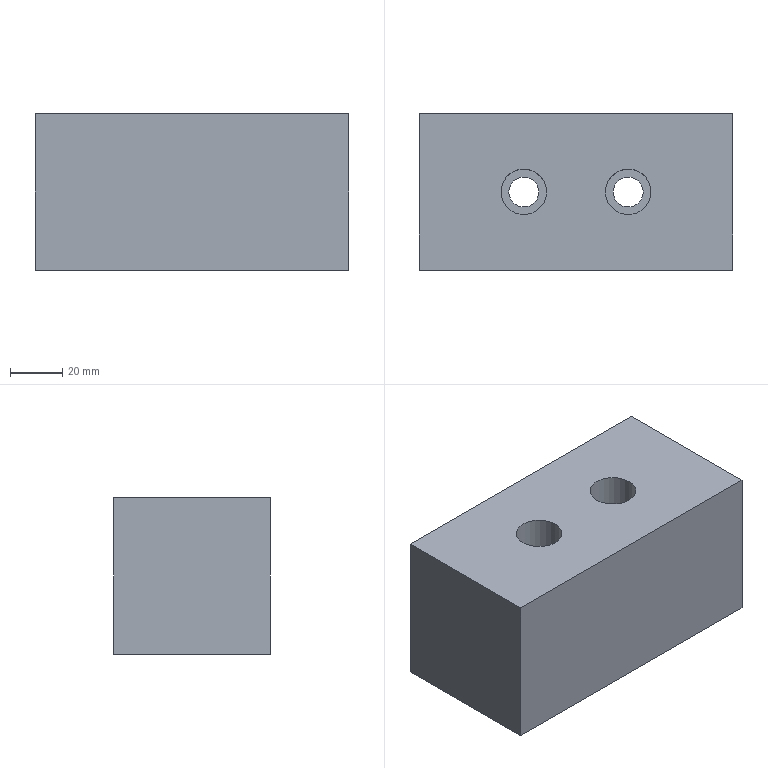Part | NX | features solid 2 | 1 solid | 12 faces | box 120 x 60 x 60 mm | volume 408603 mm3 | plane 8 | cylinder 4 | commonest cylinder face diameters 11.5 x2 17.5 x2
STEP:
#1=CARTESIAN_POINT('',(1280.,-260.,55.));
#2=VERTEX_POINT('',#1);
#3=CARTESIAN_POINT('',(1160.,-260.,55.));
#4=VERTEX_POINT('',#3);
#5=CARTESIAN_POINT('',(1295.,-260.,55.));
#6=DIRECTION('',(-1.,0.,0.));
#7=VECTOR('',#6,1000.);
#8=LINE('',#5,#7);
#9=EDGE_CURVE('',#2,#4,#8,.T.);
#10=ORIENTED_EDGE('',*,*,#9,.F.);
#11=CARTESIAN_POINT('',(1280.,-260.,-5.));
#12=VERTEX_POINT('',#11);
#13=CARTESIAN_POINT('',(1280.,-260.,-5.));
#14=DIRECTION('',(0.,0.,1.));
#15=VECTOR('',#14,1000.);
#16=LINE('',#13,#15);
#17=EDGE_CURVE('',#12,#2,#16,.T.);
#18=ORIENTED_EDGE('',*,*,#17,.F.);
#19=CARTESIAN_POINT('',(1160.,-260.,-5.));
#20=VERTEX_POINT('',#19);
#21=CARTESIAN_POINT('',(1295.,-260.,-5.));
#22=DIRECTION('',(-1.,0.,0.));
#23=VECTOR('',#22,1000.);
#24=LINE('',#21,#23);
#25=EDGE_CURVE('',#12,#20,#24,.T.);
#26=ORIENTED_EDGE('',*,*,#25,.T.);
#27=CARTESIAN_POINT('',(1160.,-260.,-5.));
#28=DIRECTION('',(0.,0.,1.));
#29=VECTOR('',#28,1000.);
#30=LINE('',#27,#29);
#31=EDGE_CURVE('',#20,#4,#30,.T.);
#32=ORIENTED_EDGE('',*,*,#31,.T.);
#33=EDGE_LOOP('',(#10,#18,#26,#32));
#34=FACE_BOUND('',#33,.T.);
#35=CARTESIAN_POINT('',(1295.,-260.,-5.));
#36=DIRECTION('',(0.,1.,0.));
#37=DIRECTION('',(0.,0.,1.));
#38=AXIS2_PLACEMENT_3D('',#35,#36,#37);
#39=PLANE('',#38);
#40=ADVANCED_FACE('',(#34),#39,.T.);
#41=CARTESIAN_POINT('',(1160.,-320.,55.));
#42=VERTEX_POINT('',#41);
#43=CARTESIAN_POINT('',(1160.,-335.,55.));
#44=DIRECTION('',(0.,1.,0.));
#45=VECTOR('',#44,1000.);
#46=LINE('',#43,#45);
#47=EDGE_CURVE('',#42,#4,#46,.T.);
#48=ORIENTED_EDGE('',*,*,#47,.T.);
#49=ORIENTED_EDGE('',*,*,#31,.F.);
#50=CARTESIAN_POINT('',(1160.,-320.,-5.));
#51=VERTEX_POINT('',#50);
#52=CARTESIAN_POINT('',(1160.,-335.,-5.));
#53=DIRECTION('',(0.,1.,0.));
#54=VECTOR('',#53,1000.);
#55=LINE('',#52,#54);
#56=EDGE_CURVE('',#51,#20,#55,.T.);
#57=ORIENTED_EDGE('',*,*,#56,.F.);
#58=CARTESIAN_POINT('',(1160.,-320.,-5.));
#59=DIRECTION('',(0.,0.,1.));
#60=VECTOR('',#59,1000.);
#61=LINE('',#58,#60);
#62=EDGE_CURVE('',#51,#42,#61,.T.);
#63=ORIENTED_EDGE('',*,*,#62,.T.);
#64=EDGE_LOOP('',(#48,#49,#57,#63));
#65=FACE_BOUND('',#64,.T.);
#66=CARTESIAN_POINT('',(1160.,-335.,-5.));
#67=DIRECTION('',(1.,0.,0.));
#68=DIRECTION('',(0.,0.,-1.));
#69=AXIS2_PLACEMENT_3D('',#66,#67,#68);
#70=PLANE('',#69);
#71=ADVANCED_FACE('',(#65),#70,.F.);
#72=CARTESIAN_POINT('',(1280.,-320.,55.));
#73=VERTEX_POINT('',#72);
#74=CARTESIAN_POINT('',(1295.,-320.,55.));
#75=DIRECTION('',(-1.,0.,0.));
#76=VECTOR('',#75,1000.);
#77=LINE('',#74,#76);
#78=EDGE_CURVE('',#73,#42,#77,.T.);
#79=ORIENTED_EDGE('',*,*,#78,.T.);
#80=ORIENTED_EDGE('',*,*,#62,.F.);
#81=CARTESIAN_POINT('',(1280.,-320.,-5.));
#82=VERTEX_POINT('',#81);
#83=CARTESIAN_POINT('',(1295.,-320.,-5.));
#84=DIRECTION('',(-1.,0.,0.));
#85=VECTOR('',#84,1000.);
#86=LINE('',#83,#85);
#87=EDGE_CURVE('',#82,#51,#86,.T.);
#88=ORIENTED_EDGE('',*,*,#87,.F.);
#89=CARTESIAN_POINT('',(1280.,-320.,-5.));
#90=DIRECTION('',(0.,0.,1.));
#91=VECTOR('',#90,1000.);
#92=LINE('',#89,#91);
#93=EDGE_CURVE('',#82,#73,#92,.T.);
#94=ORIENTED_EDGE('',*,*,#93,.T.);
#95=EDGE_LOOP('',(#79,#80,#88,#94));
#96=FACE_BOUND('',#95,.T.);
#97=CARTESIAN_POINT('',(1295.,-320.,-5.));
#98=DIRECTION('',(0.,1.,0.));
#99=DIRECTION('',(0.,0.,1.));
#100=AXIS2_PLACEMENT_3D('',#97,#98,#99);
#101=PLANE('',#100);
#102=ADVANCED_FACE('',(#96),#101,.F.);
#103=CARTESIAN_POINT('',(1280.,-335.,55.));
#104=DIRECTION('',(0.,1.,0.));
#105=VECTOR('',#104,1000.);
#106=LINE('',#103,#105);
#107=EDGE_CURVE('',#73,#2,#106,.T.);
#108=ORIENTED_EDGE('',*,*,#107,.F.);
#109=ORIENTED_EDGE('',*,*,#93,.F.);
#110=CARTESIAN_POINT('',(1280.,-335.,-5.));
#111=DIRECTION('',(0.,1.,0.));
#112=VECTOR('',#111,1000.);
#113=LINE('',#110,#112);
#114=EDGE_CURVE('',#82,#12,#113,.T.);
#115=ORIENTED_EDGE('',*,*,#114,.T.);
#116=ORIENTED_EDGE('',*,*,#17,.T.);
#117=EDGE_LOOP('',(#108,#109,#115,#116));
#118=FACE_BOUND('',#117,.T.);
#119=CARTESIAN_POINT('',(1280.,-335.,-5.));
#120=DIRECTION('',(1.,0.,0.));
#121=DIRECTION('',(0.,0.,-1.));
#122=AXIS2_PLACEMENT_3D('',#119,#120,#121);
#123=PLANE('',#122);
#124=ADVANCED_FACE('',(#118),#123,.T.);
#125=CARTESIAN_POINT('',(1194.25,-290.,-5.));
#126=VERTEX_POINT('',#125);
#127=CARTESIAN_POINT('',(1200.,-290.,-5.));
#128=DIRECTION('',(0.,0.,-1.));
#129=DIRECTION('',(-1.,0.,0.));
#130=AXIS2_PLACEMENT_3D('',#127,#128,#129);
#131=CIRCLE('',#130,5.75);
#132=EDGE_CURVE('',#126,#126,#131,.T.);
#133=ORIENTED_EDGE('',*,*,#132,.F.);
#134=EDGE_LOOP('',(#133));
#135=FACE_BOUND('',#134,.T.);
#136=CARTESIAN_POINT('',(1234.25,-290.,-5.));
#137=VERTEX_POINT('',#136);
#138=CARTESIAN_POINT('',(1240.,-290.,-5.));
#139=DIRECTION('',(0.,0.,-1.));
#140=DIRECTION('',(-1.,0.,0.));
#141=AXIS2_PLACEMENT_3D('',#138,#139,#140);
#142=CIRCLE('',#141,5.75);
#143=EDGE_CURVE('',#137,#137,#142,.T.);
#144=ORIENTED_EDGE('',*,*,#143,.F.);
#145=EDGE_LOOP('',(#144));
#146=FACE_BOUND('',#145,.T.);
#147=ORIENTED_EDGE('',*,*,#25,.F.);
#148=ORIENTED_EDGE('',*,*,#114,.F.);
#149=ORIENTED_EDGE('',*,*,#87,.T.);
#150=ORIENTED_EDGE('',*,*,#56,.T.);
#151=EDGE_LOOP('',(#147,#148,#149,#150));
#152=FACE_BOUND('',#151,.T.);
#153=CARTESIAN_POINT('',(1295.,-335.,-5.));
#154=DIRECTION('',(0.,0.,-1.));
#155=DIRECTION('',(-1.,0.,0.));
#156=AXIS2_PLACEMENT_3D('',#153,#154,#155);
#157=PLANE('',#156);
#158=ADVANCED_FACE('',(#135,#146,#152),#157,.T.);
#159=CARTESIAN_POINT('',(1191.25,-290.,55.));
#160=VERTEX_POINT('',#159);
#161=CARTESIAN_POINT('',(1200.,-290.,55.));
#162=DIRECTION('',(0.,0.,1.));
#163=DIRECTION('',(-1.,0.,0.));
#164=AXIS2_PLACEMENT_3D('',#161,#162,#163);
#165=CIRCLE('',#164,8.75);
#166=EDGE_CURVE('',#160,#160,#165,.F.);
#167=ORIENTED_EDGE('',*,*,#166,.T.);
#168=EDGE_LOOP('',(#167));
#169=FACE_BOUND('',#168,.T.);
#170=CARTESIAN_POINT('',(1231.25,-290.,55.));
#171=VERTEX_POINT('',#170);
#172=CARTESIAN_POINT('',(1240.,-290.,55.));
#173=DIRECTION('',(0.,0.,1.));
#174=DIRECTION('',(-1.,0.,0.));
#175=AXIS2_PLACEMENT_3D('',#172,#173,#174);
#176=CIRCLE('',#175,8.75);
#177=EDGE_CURVE('',#171,#171,#176,.F.);
#178=ORIENTED_EDGE('',*,*,#177,.T.);
#179=EDGE_LOOP('',(#178));
#180=FACE_BOUND('',#179,.T.);
#181=ORIENTED_EDGE('',*,*,#9,.T.);
#182=ORIENTED_EDGE('',*,*,#47,.F.);
#183=ORIENTED_EDGE('',*,*,#78,.F.);
#184=ORIENTED_EDGE('',*,*,#107,.T.);
#185=EDGE_LOOP('',(#181,#182,#183,#184));
#186=FACE_BOUND('',#185,.T.);
#187=CARTESIAN_POINT('',(1295.,-335.,55.));
#188=DIRECTION('',(0.,0.,-1.));
#189=DIRECTION('',(-1.,0.,0.));
#190=AXIS2_PLACEMENT_3D('',#187,#188,#189);
#191=PLANE('',#190);
#192=ADVANCED_FACE('',(#169,#180,#186),#191,.F.);
#193=ORIENTED_EDGE('',*,*,#143,.T.);
#194=EDGE_LOOP('',(#193));
#195=FACE_BOUND('',#194,.T.);
#196=CARTESIAN_POINT('',(1234.25,-290.,15.));
#197=VERTEX_POINT('',#196);
#198=CARTESIAN_POINT('',(1240.,-290.,15.));
#199=DIRECTION('',(0.,0.,-1.));
#200=DIRECTION('',(-1.,0.,0.));
#201=AXIS2_PLACEMENT_3D('',#198,#199,#200);
#202=CIRCLE('',#201,5.75);
#203=EDGE_CURVE('',#197,#197,#202,.T.);
#204=ORIENTED_EDGE('',*,*,#203,.F.);
#205=EDGE_LOOP('',(#204));
#206=FACE_BOUND('',#205,.T.);
#207=CARTESIAN_POINT('',(1240.,-290.,-25.));
#208=DIRECTION('',(0.,0.,-1.));
#209=DIRECTION('',(-1.,0.,0.));
#210=AXIS2_PLACEMENT_3D('',#207,#208,#209);
#211=CYLINDRICAL_SURFACE('',#210,5.75);
#212=ADVANCED_FACE('',(#195,#206),#211,.F.);
#213=ORIENTED_EDGE('',*,*,#203,.T.);
#214=EDGE_LOOP('',(#213));
#215=FACE_BOUND('',#214,.T.);
#216=CARTESIAN_POINT('',(1231.25,-290.,15.));
#217=VERTEX_POINT('',#216);
#218=CARTESIAN_POINT('',(1240.,-290.,15.));
#219=DIRECTION('',(0.,0.,-1.));
#220=DIRECTION('',(-1.,0.,0.));
#221=AXIS2_PLACEMENT_3D('',#218,#219,#220);
#222=CIRCLE('',#221,8.75);
#223=EDGE_CURVE('',#217,#217,#222,.T.);
#224=ORIENTED_EDGE('',*,*,#223,.F.);
#225=EDGE_LOOP('',(#224));
#226=FACE_BOUND('',#225,.T.);
#227=CARTESIAN_POINT('',(1240.,-290.,15.));
#228=DIRECTION('',(0.,0.,-1.));
#229=DIRECTION('',(-1.,0.,0.));
#230=AXIS2_PLACEMENT_3D('',#227,#228,#229);
#231=PLANE('',#230);
#232=ADVANCED_FACE('',(#215,#226),#231,.F.);
#233=ORIENTED_EDGE('',*,*,#223,.T.);
#234=EDGE_LOOP('',(#233));
#235=FACE_BOUND('',#234,.T.);
#236=ORIENTED_EDGE('',*,*,#177,.F.);
#237=EDGE_LOOP('',(#236));
#238=FACE_BOUND('',#237,.T.);
#239=CARTESIAN_POINT('',(1240.,-290.,65.));
#240=DIRECTION('',(0.,0.,-1.));
#241=DIRECTION('',(-1.,0.,0.));
#242=AXIS2_PLACEMENT_3D('',#239,#240,#241);
#243=CYLINDRICAL_SURFACE('',#242,8.75);
#244=ADVANCED_FACE('',(#235,#238),#243,.F.);
#245=ORIENTED_EDGE('',*,*,#132,.T.);
#246=EDGE_LOOP('',(#245));
#247=FACE_BOUND('',#246,.T.);
#248=CARTESIAN_POINT('',(1194.25,-290.,15.));
#249=VERTEX_POINT('',#248);
#250=CARTESIAN_POINT('',(1200.,-290.,15.));
#251=DIRECTION('',(0.,0.,-1.));
#252=DIRECTION('',(-1.,0.,0.));
#253=AXIS2_PLACEMENT_3D('',#250,#251,#252);
#254=CIRCLE('',#253,5.75);
#255=EDGE_CURVE('',#249,#249,#254,.T.);
#256=ORIENTED_EDGE('',*,*,#255,.F.);
#257=EDGE_LOOP('',(#256));
#258=FACE_BOUND('',#257,.T.);
#259=CARTESIAN_POINT('',(1200.,-290.,-25.));
#260=DIRECTION('',(0.,0.,-1.));
#261=DIRECTION('',(-1.,0.,0.));
#262=AXIS2_PLACEMENT_3D('',#259,#260,#261);
#263=CYLINDRICAL_SURFACE('',#262,5.75);
#264=ADVANCED_FACE('',(#247,#258),#263,.F.);
#265=ORIENTED_EDGE('',*,*,#255,.T.);
#266=EDGE_LOOP('',(#265));
#267=FACE_BOUND('',#266,.T.);
#268=CARTESIAN_POINT('',(1191.25,-290.,15.));
#269=VERTEX_POINT('',#268);
#270=CARTESIAN_POINT('',(1200.,-290.,15.));
#271=DIRECTION('',(0.,0.,-1.));
#272=DIRECTION('',(-1.,0.,0.));
#273=AXIS2_PLACEMENT_3D('',#270,#271,#272);
#274=CIRCLE('',#273,8.75);
#275=EDGE_CURVE('',#269,#269,#274,.T.);
#276=ORIENTED_EDGE('',*,*,#275,.F.);
#277=EDGE_LOOP('',(#276));
#278=FACE_BOUND('',#277,.T.);
#279=CARTESIAN_POINT('',(1200.,-290.,15.));
#280=DIRECTION('',(0.,0.,-1.));
#281=DIRECTION('',(-1.,0.,0.));
#282=AXIS2_PLACEMENT_3D('',#279,#280,#281);
#283=PLANE('',#282);
#284=ADVANCED_FACE('',(#267,#278),#283,.F.);
#285=ORIENTED_EDGE('',*,*,#275,.T.);
#286=EDGE_LOOP('',(#285));
#287=FACE_BOUND('',#286,.T.);
#288=ORIENTED_EDGE('',*,*,#166,.F.);
#289=EDGE_LOOP('',(#288));
#290=FACE_BOUND('',#289,.T.);
#291=CARTESIAN_POINT('',(1200.,-290.,65.));
#292=DIRECTION('',(0.,0.,-1.));
#293=DIRECTION('',(-1.,0.,0.));
#294=AXIS2_PLACEMENT_3D('',#291,#292,#293);
#295=CYLINDRICAL_SURFACE('',#294,8.75);
#296=ADVANCED_FACE('',(#287,#290),#295,.F.);
#297=CLOSED_SHELL('',(#40,#71,#102,#124,#158,#192,#212,#232,#244,#264,#284,#296));
#298=MANIFOLD_SOLID_BREP('',#297);
#299=(LENGTH_UNIT()NAMED_UNIT(*)SI_UNIT(.MILLI.,.METRE.));
#300=UNCERTAINTY_MEASURE_WITH_UNIT(LENGTH_MEASURE(0.00001),#299,'','');
#301=(NAMED_UNIT(*)PLANE_ANGLE_UNIT()SI_UNIT($,.RADIAN.));
#302=(NAMED_UNIT(*)SI_UNIT($,.STERADIAN.)SOLID_ANGLE_UNIT());
#303=(GEOMETRIC_REPRESENTATION_CONTEXT(3)GLOBAL_UNCERTAINTY_ASSIGNED_CONTEXT((#300))GLOBAL_UNIT_ASSIGNED_CONTEXT((#299,#301,#302))REPRESENTATION_CONTEXT('',''));
#304=ADVANCED_BREP_SHAPE_REPRESENTATION('',(#298),#303);